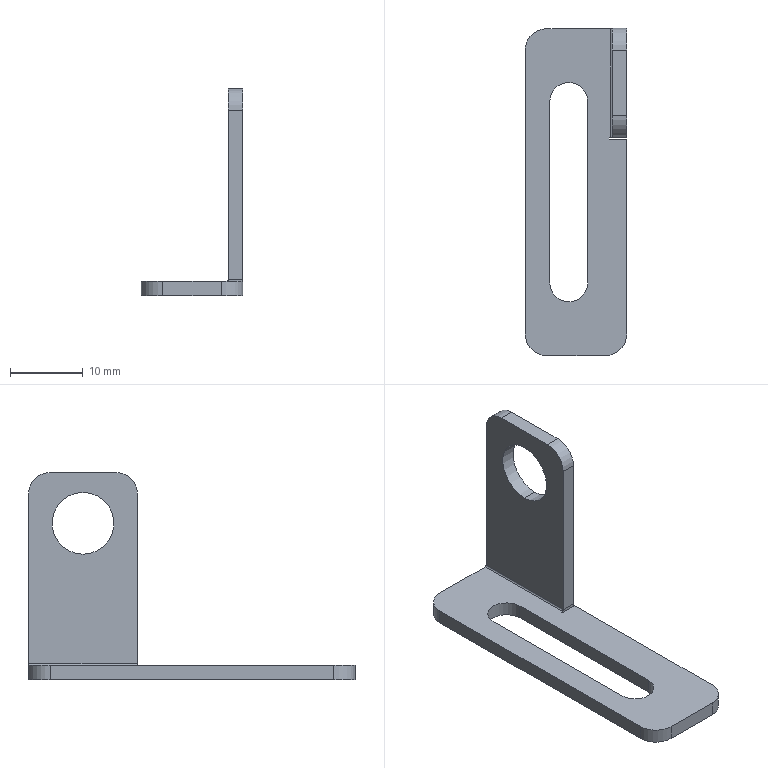Part | STEP file | ND25021-01-JDKM-02-BJ | 1 solid | 29 faces | box 14 x 45 x 28.5 mm | volume 1603 mm3 | plane 18 | cylinder 11 | commonest cylinder face diameters 6 x5 5.2 x2 8.5 x2 0.4 x1 4.4 x1